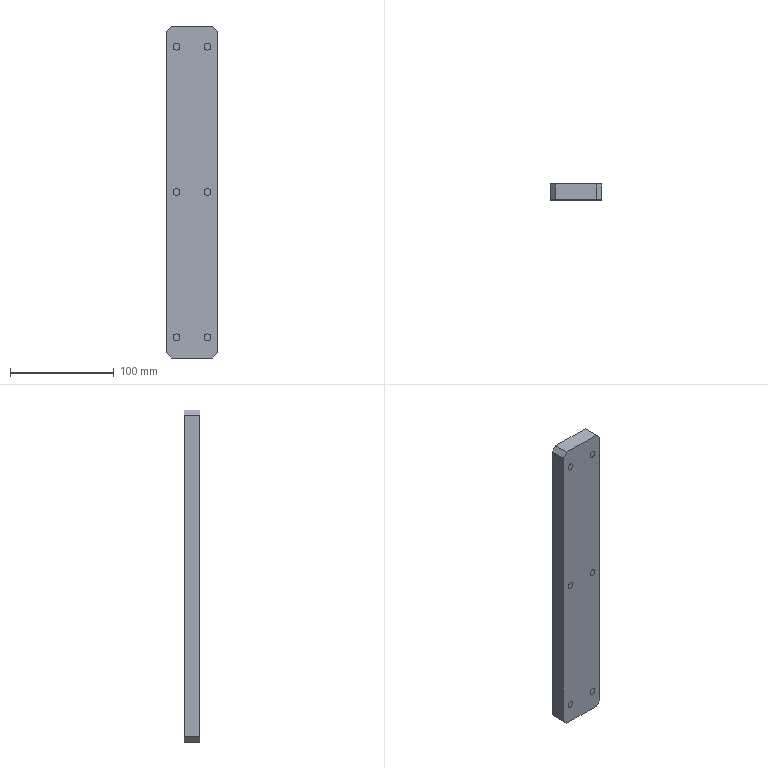Part | STEP file | CLAMP.PAD.stp | 1 solid | 46 faces | box 50 x 15.025 x 320 mm | volume 234198 mm3 | spline 24 | cylinder 12 | plane 10 | commonest cylinder face diameters 6.6 x6 11 x6